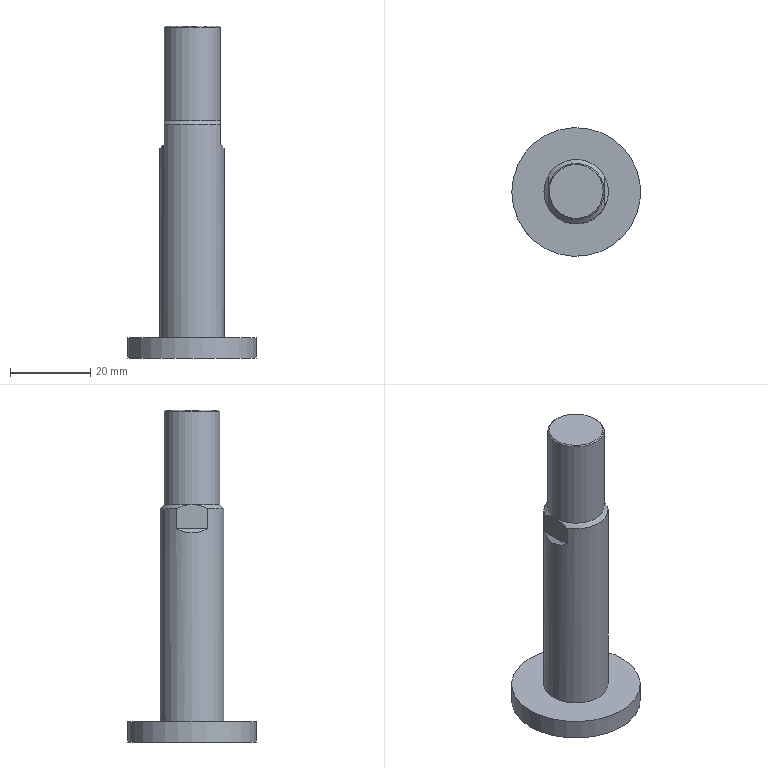Part | NX | features CDQ2B32-35DM_CQ22031Rods_32M 2 | 1 solid | 13 faces | box 32 x 32 x 82.5 mm | volume 18409 mm3 | plane 7 | cone 3 | cylinder 3 | commonest cylinder face diameters 14 x1 16 x1 32 x1
STEP:
#1=CARTESIAN_POINT('',(-6.7,0.,82.5));
#2=VERTEX_POINT('',#1);
#3=CARTESIAN_POINT('',(0.,0.,82.5));
#4=DIRECTION('',(0.,0.,-1.));
#5=DIRECTION('',(-1.,0.,0.));
#6=AXIS2_PLACEMENT_3D('',#3,#4,#5);
#7=CIRCLE('',#6,6.7);
#8=EDGE_CURVE('',#2,#2,#7,.T.);
#9=ORIENTED_EDGE('',*,*,#8,.F.);
#10=EDGE_LOOP('',(#9));
#11=FACE_BOUND('',#10,.T.);
#12=CARTESIAN_POINT('',(0.,0.,82.5));
#13=DIRECTION('',(0.,0.,1.));
#14=DIRECTION('',(1.,0.,0.));
#15=AXIS2_PLACEMENT_3D('',#12,#13,#14);
#16=PLANE('',#15);
#17=ADVANCED_FACE('',(#11),#16,.T.);
#18=CARTESIAN_POINT('',(-16.,0.,0.));
#19=VERTEX_POINT('',#18);
#20=CARTESIAN_POINT('',(0.,0.,0.));
#21=DIRECTION('',(0.,0.,-1.));
#22=DIRECTION('',(-1.,0.,0.));
#23=AXIS2_PLACEMENT_3D('',#20,#21,#22);
#24=CIRCLE('',#23,16.);
#25=EDGE_CURVE('',#19,#19,#24,.F.);
#26=ORIENTED_EDGE('',*,*,#25,.F.);
#27=EDGE_LOOP('',(#26));
#28=FACE_BOUND('',#27,.T.);
#29=CARTESIAN_POINT('',(0.,0.,0.));
#30=DIRECTION('',(0.,0.,1.));
#31=DIRECTION('',(1.,0.,0.));
#32=AXIS2_PLACEMENT_3D('',#29,#30,#31);
#33=PLANE('',#32);
#34=ADVANCED_FACE('',(#28),#33,.F.);
#35=CARTESIAN_POINT('',(-7.,0.,82.2));
#36=VERTEX_POINT('',#35);
#37=CARTESIAN_POINT('',(0.,0.,82.2));
#38=DIRECTION('',(0.,0.,-1.));
#39=DIRECTION('',(-1.,0.,0.));
#40=AXIS2_PLACEMENT_3D('',#37,#38,#39);
#41=CIRCLE('',#40,7.);
#42=EDGE_CURVE('',#36,#36,#41,.T.);
#43=ORIENTED_EDGE('',*,*,#42,.F.);
#44=EDGE_LOOP('',(#43));
#45=FACE_BOUND('',#44,.T.);
#46=ORIENTED_EDGE('',*,*,#8,.T.);
#47=EDGE_LOOP('',(#46));
#48=FACE_BOUND('',#47,.T.);
#49=CARTESIAN_POINT('',(0.,0.,82.2));
#50=DIRECTION('',(0.,0.,-1.));
#51=DIRECTION('',(-1.,0.,0.));
#52=AXIS2_PLACEMENT_3D('',#49,#50,#51);
#53=CONICAL_SURFACE('',#52,7.,0.7854);
#54=ADVANCED_FACE('',(#45,#48),#53,.T.);
#55=ORIENTED_EDGE('',*,*,#25,.T.);
#56=EDGE_LOOP('',(#55));
#57=FACE_BOUND('',#56,.T.);
#58=CARTESIAN_POINT('',(-16.,0.,5.));
#59=VERTEX_POINT('',#58);
#60=CARTESIAN_POINT('',(0.,0.,5.));
#61=DIRECTION('',(0.,0.,-1.));
#62=DIRECTION('',(-1.,0.,0.));
#63=AXIS2_PLACEMENT_3D('',#60,#61,#62);
#64=CIRCLE('',#63,16.);
#65=EDGE_CURVE('',#59,#59,#64,.F.);
#66=ORIENTED_EDGE('',*,*,#65,.F.);
#67=EDGE_LOOP('',(#66));
#68=FACE_BOUND('',#67,.T.);
#69=CARTESIAN_POINT('',(0.,0.,5.));
#70=DIRECTION('',(0.,0.,-1.));
#71=DIRECTION('',(-1.,0.,0.));
#72=AXIS2_PLACEMENT_3D('',#69,#70,#71);
#73=CYLINDRICAL_SURFACE('',#72,16.);
#74=ADVANCED_FACE('',(#57,#68),#73,.T.);
#75=CARTESIAN_POINT('',(7.,0.,59.));
#76=VERTEX_POINT('',#75);
#77=CARTESIAN_POINT('',(-7.,0.,59.));
#78=VERTEX_POINT('',#77);
#79=CARTESIAN_POINT('',(0.,0.,59.));
#80=DIRECTION('',(0.,0.,-1.));
#81=DIRECTION('',(-1.,0.,0.));
#82=AXIS2_PLACEMENT_3D('',#79,#80,#81);
#83=CIRCLE('',#82,7.);
#84=EDGE_CURVE('',#76,#78,#83,.T.);
#85=ORIENTED_EDGE('',*,*,#84,.F.);
#86=CARTESIAN_POINT('',(0.,0.,59.));
#87=DIRECTION('',(0.,0.,-1.));
#88=DIRECTION('',(-1.,0.,0.));
#89=AXIS2_PLACEMENT_3D('',#86,#87,#88);
#90=CIRCLE('',#89,7.);
#91=EDGE_CURVE('',#78,#76,#90,.T.);
#92=ORIENTED_EDGE('',*,*,#91,.F.);
#93=EDGE_LOOP('',(#85,#92));
#94=FACE_BOUND('',#93,.T.);
#95=ORIENTED_EDGE('',*,*,#42,.T.);
#96=EDGE_LOOP('',(#95));
#97=FACE_BOUND('',#96,.T.);
#98=CARTESIAN_POINT('',(0.,0.,82.5));
#99=DIRECTION('',(0.,0.,-1.));
#100=DIRECTION('',(-1.,0.,0.));
#101=AXIS2_PLACEMENT_3D('',#98,#99,#100);
#102=CYLINDRICAL_SURFACE('',#101,7.);
#103=ADVANCED_FACE('',(#94,#97),#102,.T.);
#104=CARTESIAN_POINT('',(7.,-3.873,58.));
#105=VERTEX_POINT('',#104);
#106=CARTESIAN_POINT('',(7.,-3.873,58.));
#107=CARTESIAN_POINT('',(7.,-2.655,58.59));
#108=CARTESIAN_POINT('',(7.,-1.365,59.));
#109=CARTESIAN_POINT('',(7.,0.,59.));
#110=B_SPLINE_CURVE_WITH_KNOTS('',3,(#106,#107,#108,#109),.UNSPECIFIED.,.F.,.F.,(4,4),(0.,0.004002),.UNSPECIFIED.);
#111=EDGE_CURVE('',#105,#76,#110,.T.);
#112=ORIENTED_EDGE('',*,*,#111,.T.);
#113=ORIENTED_EDGE('',*,*,#84,.T.);
#114=CARTESIAN_POINT('',(-7.,-3.873,58.));
#115=VERTEX_POINT('',#114);
#116=CARTESIAN_POINT('',(-7.,0.,59.));
#117=CARTESIAN_POINT('',(-7.,-1.356,59.));
#118=CARTESIAN_POINT('',(-7.,-2.657,58.589));
#119=CARTESIAN_POINT('',(-7.,-3.873,58.));
#120=B_SPLINE_CURVE_WITH_KNOTS('',3,(#116,#117,#118,#119),.UNSPECIFIED.,.F.,.F.,(4,4),(0.,0.004009),.UNSPECIFIED.);
#121=EDGE_CURVE('',#78,#115,#120,.T.);
#122=ORIENTED_EDGE('',*,*,#121,.T.);
#123=CARTESIAN_POINT('',(0.,0.,58.));
#124=DIRECTION('',(0.,0.,-1.));
#125=DIRECTION('',(-1.,0.,0.));
#126=AXIS2_PLACEMENT_3D('',#123,#124,#125);
#127=CIRCLE('',#126,8.);
#128=EDGE_CURVE('',#105,#115,#127,.T.);
#129=ORIENTED_EDGE('',*,*,#128,.F.);
#130=EDGE_LOOP('',(#112,#113,#122,#129));
#131=FACE_BOUND('',#130,.T.);
#132=CARTESIAN_POINT('',(0.,0.,58.));
#133=DIRECTION('',(0.,0.,-1.));
#134=DIRECTION('',(0.,1.,0.));
#135=AXIS2_PLACEMENT_3D('',#132,#133,#134);
#136=CONICAL_SURFACE('',#135,8.,0.7854);
#137=ADVANCED_FACE('',(#131),#136,.T.);
#138=CARTESIAN_POINT('',(7.,3.873,53.));
#139=VERTEX_POINT('',#138);
#140=CARTESIAN_POINT('',(7.,-3.873,53.));
#141=VERTEX_POINT('',#140);
#142=CARTESIAN_POINT('',(7.,7.5,53.));
#143=DIRECTION('',(0.,1.,0.));
#144=VECTOR('',#143,1000.);
#145=LINE('',#142,#144);
#146=EDGE_CURVE('',#139,#141,#145,.F.);
#147=ORIENTED_EDGE('',*,*,#146,.T.);
#148=CARTESIAN_POINT('',(0.,0.,60.));
#149=DIRECTION('',(-0.7071,0.,-0.7071));
#150=DIRECTION('',(0.7071,0.,-0.7071));
#151=AXIS2_PLACEMENT_3D('',#148,#149,#150);
#152=ELLIPSE('',#151,11.314,8.);
#153=EDGE_CURVE('',#139,#141,#152,.T.);
#154=ORIENTED_EDGE('',*,*,#153,.F.);
#155=EDGE_LOOP('',(#147,#154));
#156=FACE_BOUND('',#155,.T.);
#157=CARTESIAN_POINT('',(8.,7.5,52.));
#158=DIRECTION('',(-0.7071,0.,-0.7071));
#159=DIRECTION('',(-0.7071,0.,0.7071));
#160=AXIS2_PLACEMENT_3D('',#157,#158,#159);
#161=PLANE('',#160);
#162=ADVANCED_FACE('',(#156),#161,.F.);
#163=CARTESIAN_POINT('',(-8.,0.,5.));
#164=VERTEX_POINT('',#163);
#165=CARTESIAN_POINT('',(0.,0.,5.));
#166=DIRECTION('',(0.,0.,-1.));
#167=DIRECTION('',(-1.,0.,0.));
#168=AXIS2_PLACEMENT_3D('',#165,#166,#167);
#169=CIRCLE('',#168,8.);
#170=EDGE_CURVE('',#164,#164,#169,.F.);
#171=ORIENTED_EDGE('',*,*,#170,.F.);
#172=EDGE_LOOP('',(#171));
#173=FACE_BOUND('',#172,.T.);
#174=ORIENTED_EDGE('',*,*,#65,.T.);
#175=EDGE_LOOP('',(#174));
#176=FACE_BOUND('',#175,.T.);
#177=CARTESIAN_POINT('',(0.,0.,5.));
#178=DIRECTION('',(0.,0.,1.));
#179=DIRECTION('',(1.,0.,0.));
#180=AXIS2_PLACEMENT_3D('',#177,#178,#179);
#181=PLANE('',#180);
#182=ADVANCED_FACE('',(#173,#176),#181,.T.);
#183=CARTESIAN_POINT('',(-7.,-3.873,53.));
#184=VERTEX_POINT('',#183);
#185=CARTESIAN_POINT('',(-7.,3.873,53.));
#186=VERTEX_POINT('',#185);
#187=CARTESIAN_POINT('',(-7.,7.5,53.));
#188=DIRECTION('',(0.,1.,0.));
#189=VECTOR('',#188,1000.);
#190=LINE('',#187,#189);
#191=EDGE_CURVE('',#184,#186,#190,.T.);
#192=ORIENTED_EDGE('',*,*,#191,.T.);
#193=CARTESIAN_POINT('',(0.,0.,60.));
#194=DIRECTION('',(-0.7071,0.,0.7071));
#195=DIRECTION('',(-0.7071,0.,-0.7071));
#196=AXIS2_PLACEMENT_3D('',#193,#194,#195);
#197=ELLIPSE('',#196,11.314,8.);
#198=EDGE_CURVE('',#184,#186,#197,.F.);
#199=ORIENTED_EDGE('',*,*,#198,.F.);
#200=EDGE_LOOP('',(#192,#199));
#201=FACE_BOUND('',#200,.T.);
#202=CARTESIAN_POINT('',(-8.,7.5,52.));
#203=DIRECTION('',(-0.7071,0.,0.7071));
#204=DIRECTION('',(0.7071,0.,0.7071));
#205=AXIS2_PLACEMENT_3D('',#202,#203,#204);
#206=PLANE('',#205);
#207=ADVANCED_FACE('',(#201),#206,.T.);
#208=ORIENTED_EDGE('',*,*,#191,.F.);
#209=CARTESIAN_POINT('',(-7.,-3.873,52.));
#210=DIRECTION('',(0.,0.,-1.));
#211=VECTOR('',#210,1000.);
#212=LINE('',#209,#211);
#213=EDGE_CURVE('',#115,#184,#212,.T.);
#214=ORIENTED_EDGE('',*,*,#213,.F.);
#215=ORIENTED_EDGE('',*,*,#121,.F.);
#216=CARTESIAN_POINT('',(-7.,3.873,58.));
#217=VERTEX_POINT('',#216);
#218=CARTESIAN_POINT('',(-7.,3.873,58.));
#219=CARTESIAN_POINT('',(-7.,2.655,58.59));
#220=CARTESIAN_POINT('',(-7.,1.365,59.));
#221=CARTESIAN_POINT('',(-7.,0.,59.));
#222=B_SPLINE_CURVE_WITH_KNOTS('',3,(#218,#219,#220,#221),.UNSPECIFIED.,.F.,.F.,(4,4),(0.,0.004002),.UNSPECIFIED.);
#223=EDGE_CURVE('',#217,#78,#222,.T.);
#224=ORIENTED_EDGE('',*,*,#223,.F.);
#225=CARTESIAN_POINT('',(-7.,3.873,81.627));
#226=DIRECTION('',(0.,0.,-1.));
#227=VECTOR('',#226,1000.);
#228=LINE('',#225,#227);
#229=EDGE_CURVE('',#186,#217,#228,.F.);
#230=ORIENTED_EDGE('',*,*,#229,.F.);
#231=EDGE_LOOP('',(#208,#214,#215,#224,#230));
#232=FACE_BOUND('',#231,.T.);
#233=CARTESIAN_POINT('',(-7.,7.5,52.));
#234=DIRECTION('',(1.,0.,0.));
#235=DIRECTION('',(0.,0.,-1.));
#236=AXIS2_PLACEMENT_3D('',#233,#234,#235);
#237=PLANE('',#236);
#238=ADVANCED_FACE('',(#232),#237,.F.);
#239=CARTESIAN_POINT('',(7.,3.873,58.));
#240=VERTEX_POINT('',#239);
#241=CARTESIAN_POINT('',(7.,0.,59.));
#242=CARTESIAN_POINT('',(7.,1.356,59.));
#243=CARTESIAN_POINT('',(7.,2.657,58.589));
#244=CARTESIAN_POINT('',(7.,3.873,58.));
#245=B_SPLINE_CURVE_WITH_KNOTS('',3,(#241,#242,#243,#244),.UNSPECIFIED.,.F.,.F.,(4,4),(0.,0.004009),.UNSPECIFIED.);
#246=EDGE_CURVE('',#76,#240,#245,.T.);
#247=ORIENTED_EDGE('',*,*,#246,.T.);
#248=CARTESIAN_POINT('',(0.,0.,58.));
#249=DIRECTION('',(0.,0.,-1.));
#250=DIRECTION('',(-1.,0.,0.));
#251=AXIS2_PLACEMENT_3D('',#248,#249,#250);
#252=CIRCLE('',#251,8.);
#253=EDGE_CURVE('',#217,#240,#252,.T.);
#254=ORIENTED_EDGE('',*,*,#253,.F.);
#255=ORIENTED_EDGE('',*,*,#223,.T.);
#256=ORIENTED_EDGE('',*,*,#91,.T.);
#257=EDGE_LOOP('',(#247,#254,#255,#256));
#258=FACE_BOUND('',#257,.T.);
#259=CARTESIAN_POINT('',(0.,0.,58.));
#260=DIRECTION('',(0.,0.,-1.));
#261=DIRECTION('',(0.,1.,0.));
#262=AXIS2_PLACEMENT_3D('',#259,#260,#261);
#263=CONICAL_SURFACE('',#262,8.,0.7854);
#264=ADVANCED_FACE('',(#258),#263,.T.);
#265=ORIENTED_EDGE('',*,*,#146,.F.);
#266=CARTESIAN_POINT('',(7.,3.873,81.627));
#267=DIRECTION('',(0.,0.,-1.));
#268=VECTOR('',#267,1000.);
#269=LINE('',#266,#268);
#270=EDGE_CURVE('',#240,#139,#269,.T.);
#271=ORIENTED_EDGE('',*,*,#270,.F.);
#272=ORIENTED_EDGE('',*,*,#246,.F.);
#273=ORIENTED_EDGE('',*,*,#111,.F.);
#274=CARTESIAN_POINT('',(7.,-3.873,52.));
#275=DIRECTION('',(0.,0.,1.));
#276=VECTOR('',#275,1000.);
#277=LINE('',#274,#276);
#278=EDGE_CURVE('',#141,#105,#277,.T.);
#279=ORIENTED_EDGE('',*,*,#278,.F.);
#280=EDGE_LOOP('',(#265,#271,#272,#273,#279));
#281=FACE_BOUND('',#280,.T.);
#282=CARTESIAN_POINT('',(7.,7.5,52.));
#283=DIRECTION('',(-1.,0.,0.));
#284=DIRECTION('',(0.,0.,1.));
#285=AXIS2_PLACEMENT_3D('',#282,#283,#284);
#286=PLANE('',#285);
#287=ADVANCED_FACE('',(#281),#286,.F.);
#288=ORIENTED_EDGE('',*,*,#170,.T.);
#289=EDGE_LOOP('',(#288));
#290=FACE_BOUND('',#289,.T.);
#291=ORIENTED_EDGE('',*,*,#253,.T.);
#292=ORIENTED_EDGE('',*,*,#270,.T.);
#293=ORIENTED_EDGE('',*,*,#153,.T.);
#294=ORIENTED_EDGE('',*,*,#278,.T.);
#295=ORIENTED_EDGE('',*,*,#128,.T.);
#296=ORIENTED_EDGE('',*,*,#213,.T.);
#297=ORIENTED_EDGE('',*,*,#198,.T.);
#298=ORIENTED_EDGE('',*,*,#229,.T.);
#299=EDGE_LOOP('',(#291,#292,#293,#294,#295,#296,#297,#298));
#300=FACE_BOUND('',#299,.T.);
#301=CARTESIAN_POINT('',(0.,0.,81.627));
#302=DIRECTION('',(0.,0.,-1.));
#303=DIRECTION('',(-1.,0.,0.));
#304=AXIS2_PLACEMENT_3D('',#301,#302,#303);
#305=CYLINDRICAL_SURFACE('',#304,8.);
#306=ADVANCED_FACE('',(#290,#300),#305,.T.);
#307=CLOSED_SHELL('',(#17,#34,#54,#74,#103,#137,#162,#182,#207,#238,#264,#287,#306));
#308=MANIFOLD_SOLID_BREP('',#307);
#309=(LENGTH_UNIT()NAMED_UNIT(*)SI_UNIT(.MILLI.,.METRE.));
#310=UNCERTAINTY_MEASURE_WITH_UNIT(LENGTH_MEASURE(0.0508),#309,'','');
#311=(NAMED_UNIT(*)PLANE_ANGLE_UNIT()SI_UNIT($,.RADIAN.));
#312=(NAMED_UNIT(*)SI_UNIT($,.STERADIAN.)SOLID_ANGLE_UNIT());
#313=(GEOMETRIC_REPRESENTATION_CONTEXT(3)GLOBAL_UNCERTAINTY_ASSIGNED_CONTEXT((#310))GLOBAL_UNIT_ASSIGNED_CONTEXT((#309,#311,#312))REPRESENTATION_CONTEXT('',''));
#314=ADVANCED_BREP_SHAPE_REPRESENTATION('',(#308),#313);